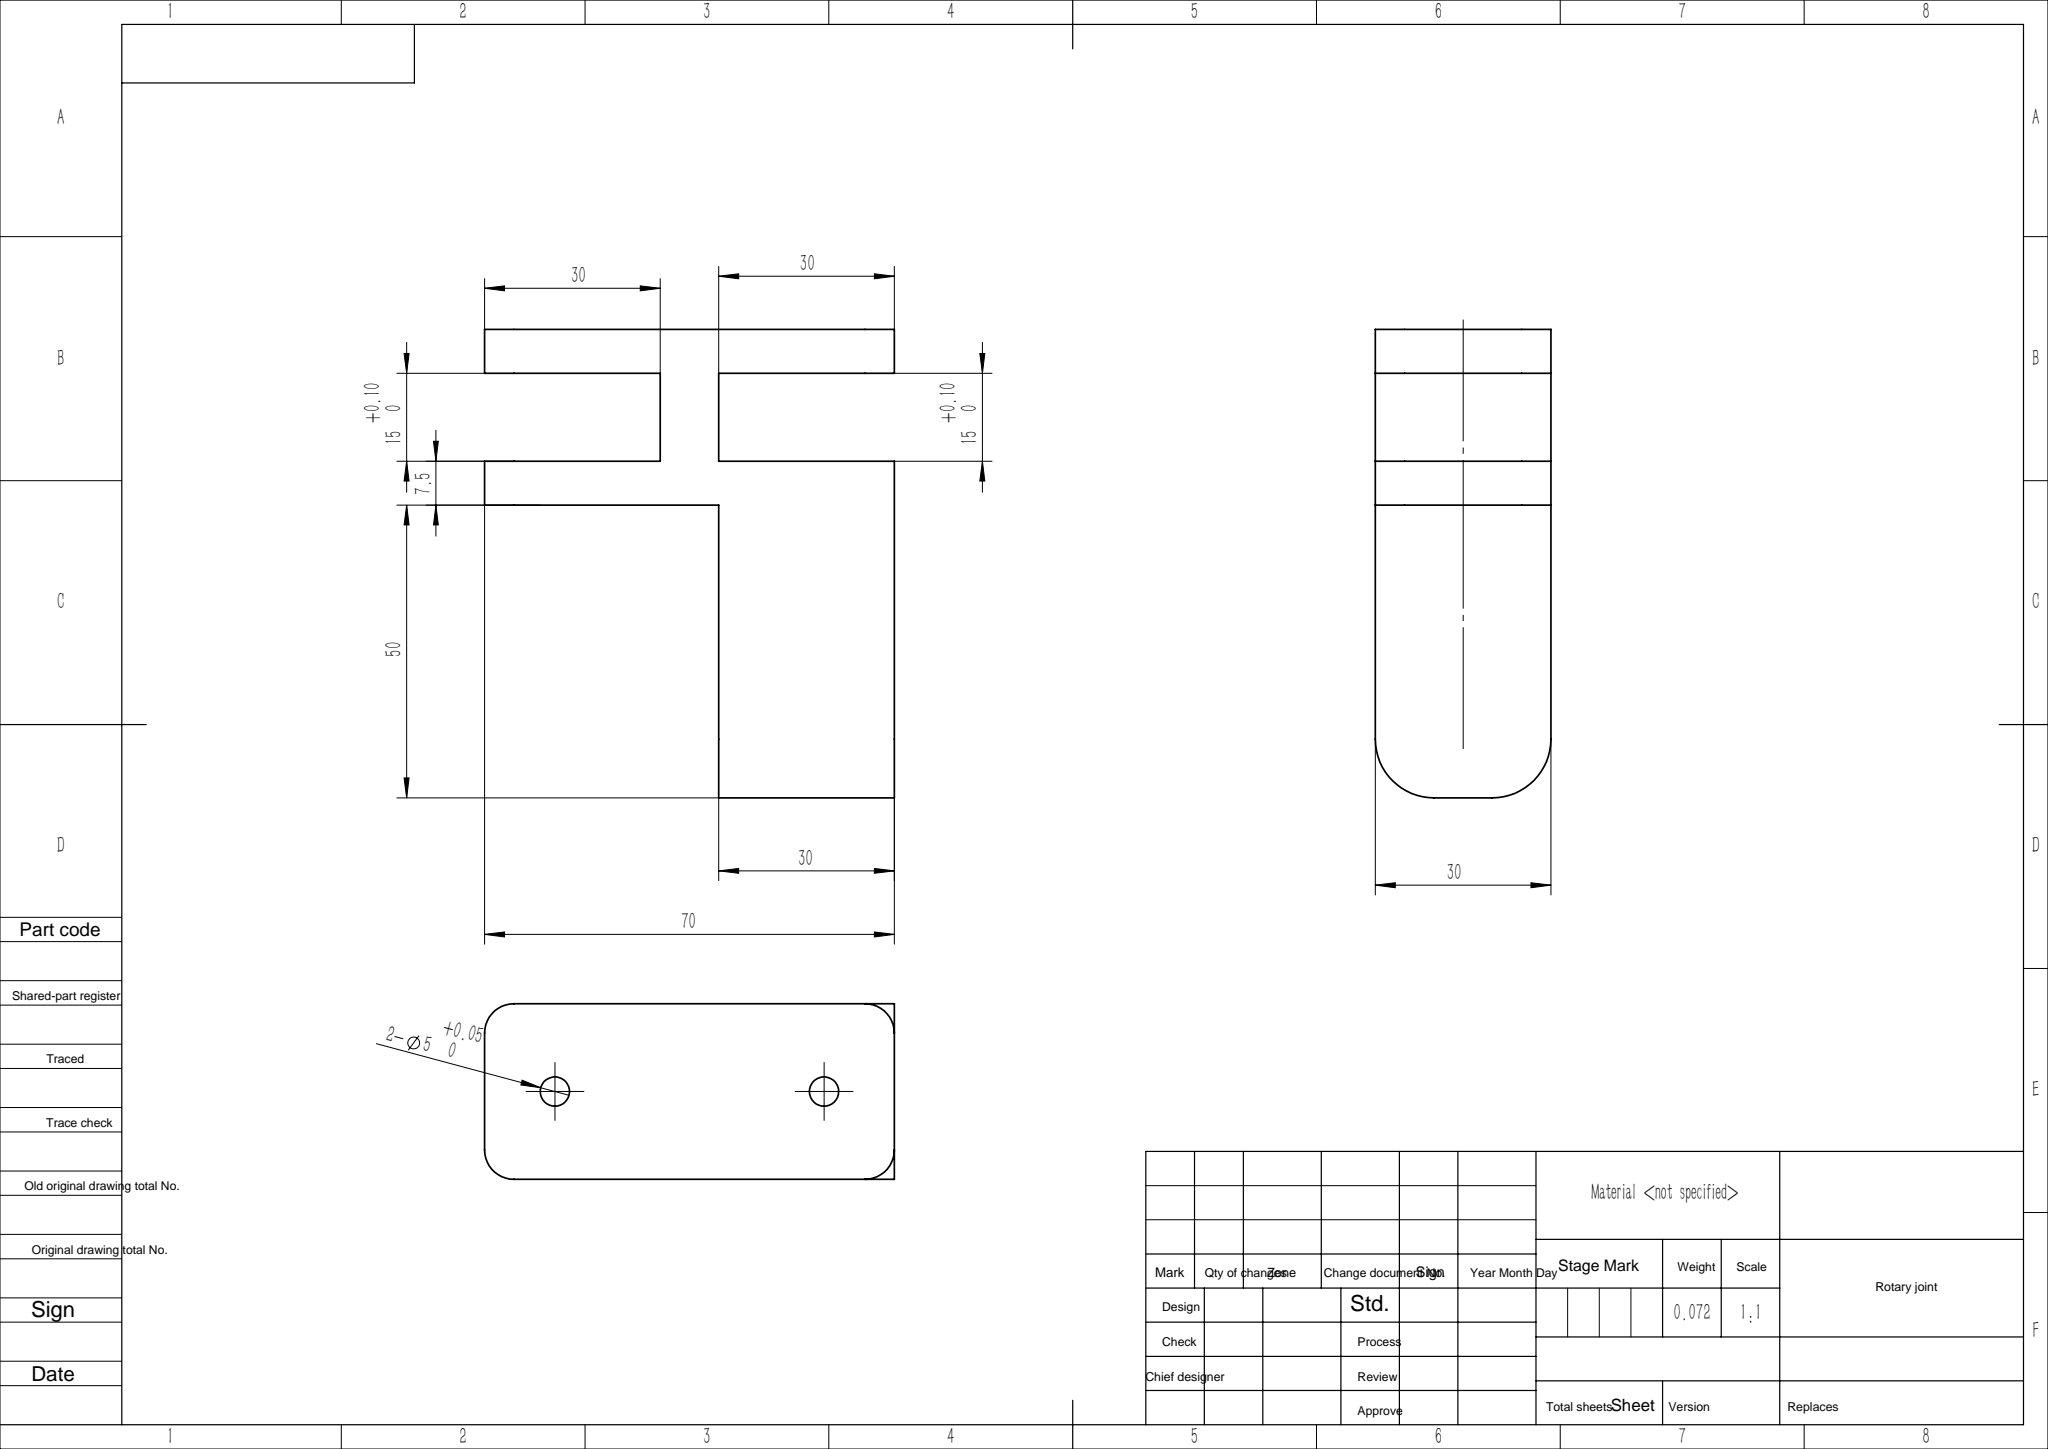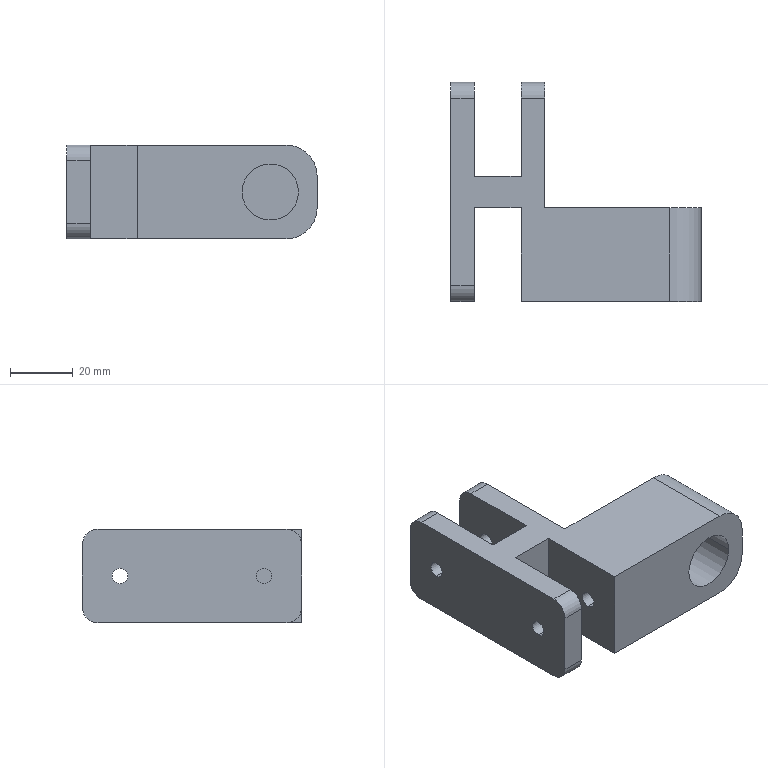Part | SolidWorks | features ICE 3, Fillet 2, Extrusion 1 | 1 solid | 36 faces | box 80 x 70 x 30 mm | volume 72177 mm3 | cylinder 18 | plane 18 | commonest cylinder face diameters 5 x8 10 x6 18 x2 20 x2